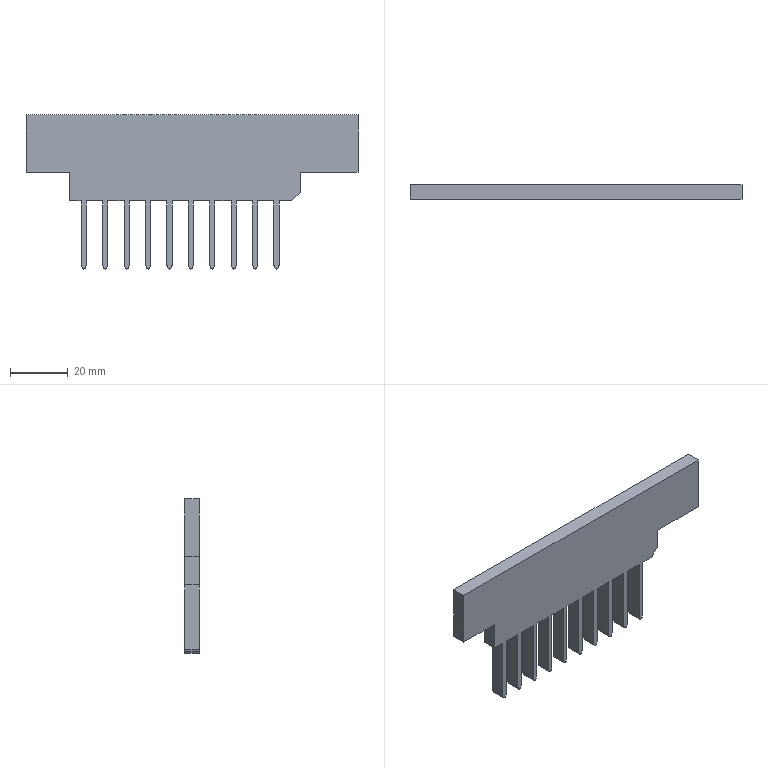Part | STEP file | 200 mesh_id2014 | 1 solid | 91 faces | box 115.071 x 4.98 x 53.4 mm | volume 17394 mm3 | plane 81 | cylinder 10 | commonest cylinder face diameters 1.211 x10